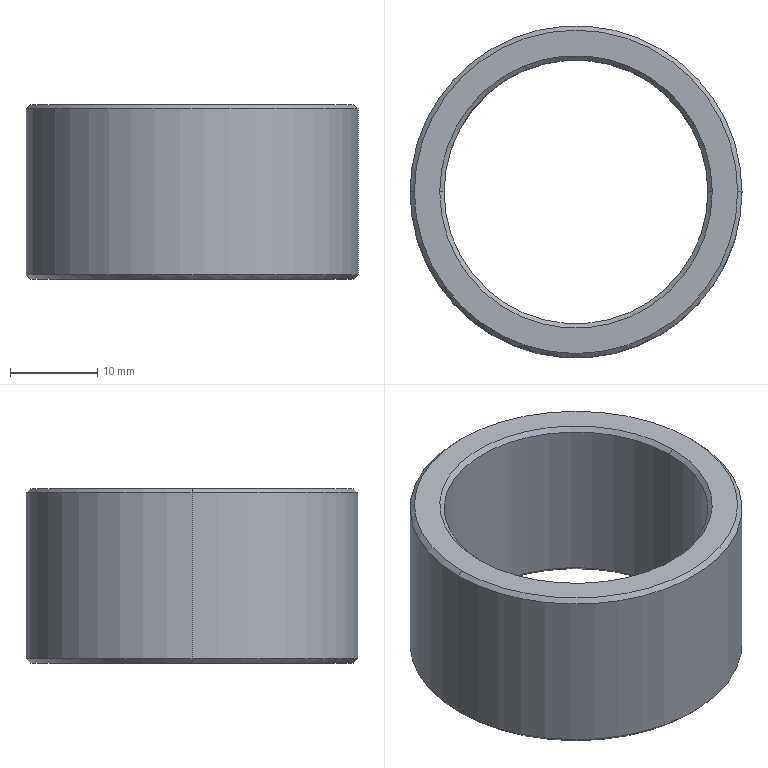Part | STEP file | 2097 Shaft bearing | 1 solid | 14 faces | box 38 x 38 x 20 mm | volume 8302 mm3 | cone 8 | cylinder 4 | plane 2 | commonest cylinder face diameters 30.2 x2 38 x2
STEP:
#1=CARTESIAN_POINT('',(0.,0.,0.));
#2=DIRECTION('',(0.,0.,1.));
#3=DIRECTION('',(1.,0.,0.));
#4=AXIS2_PLACEMENT_3D('',#1,#2,#3);
#5=CARTESIAN_POINT('',(18.5,0.,20.));
#6=VERTEX_POINT('',#5);
#7=CARTESIAN_POINT('',(-18.5,0.,20.));
#8=VERTEX_POINT('',#7);
#9=CARTESIAN_POINT('',(0.,0.,20.));
#10=DIRECTION('',(0.,0.,1.));
#11=DIRECTION('',(1.,0.,0.));
#12=AXIS2_PLACEMENT_3D('',#9,#10,#11);
#13=CIRCLE('',#12,18.5);
#14=CARTESIAN_POINT('',(0.,0.,20.));
#15=DIRECTION('',(0.,0.,-1.));
#16=DIRECTION('',(-1.,0.,0.));
#17=AXIS2_PLACEMENT_3D('',#14,#15,#16);
#18=CONICAL_SURFACE('',#17,18.5,0.7854);
#19=CARTESIAN_POINT('',(3.142,0.));
#20=DIRECTION('',(-1.,0.));
#21=VECTOR('',#20,1.);
#22=LINE('',#19,#21);
#23=(GEOMETRIC_REPRESENTATION_CONTEXT(2)PARAMETRIC_REPRESENTATION_CONTEXT()REPRESENTATION_CONTEXT('',''));
#24=DEFINITIONAL_REPRESENTATION('',(#22),#23);
#25=PCURVE('',#18,#24);
#26=CARTESIAN_POINT('',(0.,0.,20.));
#27=DIRECTION('',(0.,0.,1.));
#28=DIRECTION('',(1.,0.,0.));
#29=AXIS2_PLACEMENT_3D('',#26,#27,#28);
#30=PLANE('',#29);
#31=CARTESIAN_POINT('',(0.,0.));
#32=DIRECTION('',(1.,0.));
#33=AXIS2_PLACEMENT_2D('',#31,#32);
#34=CIRCLE('',#33,18.5);
#35=(GEOMETRIC_REPRESENTATION_CONTEXT(2)PARAMETRIC_REPRESENTATION_CONTEXT()REPRESENTATION_CONTEXT('',''));
#36=DEFINITIONAL_REPRESENTATION('',(#34),#35);
#37=PCURVE('',#30,#36);
#38=SURFACE_CURVE('',#13,(#25,#37),.PCURVE_S1.);
#39=EDGE_CURVE('',#6,#8,#38,.T.);
#40=ORIENTED_EDGE('',*,*,#39,.F.);
#41=CARTESIAN_POINT('',(19.,0.,19.5));
#42=VERTEX_POINT('',#41);
#43=CARTESIAN_POINT('',(18.5,0.,20.));
#44=DIRECTION('',(0.7071,0.,-0.7071));
#45=VECTOR('',#44,1.);
#46=LINE('',#43,#45);
#47=CARTESIAN_POINT('',(3.142,0.));
#48=DIRECTION('',(0.,1.));
#49=VECTOR('',#48,1.);
#50=LINE('',#47,#49);
#51=(GEOMETRIC_REPRESENTATION_CONTEXT(2)PARAMETRIC_REPRESENTATION_CONTEXT()REPRESENTATION_CONTEXT('',''));
#52=DEFINITIONAL_REPRESENTATION('',(#50),#51);
#53=PCURVE('',#18,#52);
#54=CARTESIAN_POINT('',(0.,0.,20.));
#55=DIRECTION('',(0.,0.,-1.));
#56=DIRECTION('',(-1.,0.,0.));
#57=AXIS2_PLACEMENT_3D('',#54,#55,#56);
#58=CONICAL_SURFACE('',#57,18.5,0.7854);
#59=CARTESIAN_POINT('',(3.142,0.));
#60=DIRECTION('',(0.,1.));
#61=VECTOR('',#60,1.);
#62=LINE('',#59,#61);
#63=(GEOMETRIC_REPRESENTATION_CONTEXT(2)PARAMETRIC_REPRESENTATION_CONTEXT()REPRESENTATION_CONTEXT('',''));
#64=DEFINITIONAL_REPRESENTATION('',(#62),#63);
#65=PCURVE('',#58,#64);
#66=SURFACE_CURVE('',#46,(#53,#65),.PCURVE_S1.);
#67=EDGE_CURVE('',#6,#42,#66,.T.);
#68=ORIENTED_EDGE('',*,*,#67,.T.);
#69=CARTESIAN_POINT('',(-19.,0.,19.5));
#70=VERTEX_POINT('',#69);
#71=CARTESIAN_POINT('',(0.,0.,19.5));
#72=DIRECTION('',(0.,0.,-1.));
#73=DIRECTION('',(1.,0.,0.));
#74=AXIS2_PLACEMENT_3D('',#71,#72,#73);
#75=CIRCLE('',#74,19.);
#76=CARTESIAN_POINT('',(-3.142,0.5));
#77=DIRECTION('',(1.,0.));
#78=VECTOR('',#77,1.);
#79=LINE('',#76,#78);
#80=(GEOMETRIC_REPRESENTATION_CONTEXT(2)PARAMETRIC_REPRESENTATION_CONTEXT()REPRESENTATION_CONTEXT('',''));
#81=DEFINITIONAL_REPRESENTATION('',(#79),#80);
#82=PCURVE('',#18,#81);
#83=CARTESIAN_POINT('',(0.,0.,20.));
#84=DIRECTION('',(0.,0.,-1.));
#85=DIRECTION('',(-1.,0.,0.));
#86=AXIS2_PLACEMENT_3D('',#83,#84,#85);
#87=CYLINDRICAL_SURFACE('',#86,19.);
#88=CARTESIAN_POINT('',(-3.142,0.5));
#89=DIRECTION('',(1.,0.));
#90=VECTOR('',#89,1.);
#91=LINE('',#88,#90);
#92=(GEOMETRIC_REPRESENTATION_CONTEXT(2)PARAMETRIC_REPRESENTATION_CONTEXT()REPRESENTATION_CONTEXT('',''));
#93=DEFINITIONAL_REPRESENTATION('',(#91),#92);
#94=PCURVE('',#87,#93);
#95=SURFACE_CURVE('',#75,(#82,#94),.PCURVE_S1.);
#96=EDGE_CURVE('',#70,#42,#95,.T.);
#97=ORIENTED_EDGE('',*,*,#96,.F.);
#98=CARTESIAN_POINT('',(-18.5,0.,20.));
#99=DIRECTION('',(-0.7071,0.,-0.7071));
#100=VECTOR('',#99,1.);
#101=LINE('',#98,#100);
#102=CARTESIAN_POINT('',(0.,0.));
#103=DIRECTION('',(0.,1.));
#104=VECTOR('',#103,1.);
#105=LINE('',#102,#104);
#106=(GEOMETRIC_REPRESENTATION_CONTEXT(2)PARAMETRIC_REPRESENTATION_CONTEXT()REPRESENTATION_CONTEXT('',''));
#107=DEFINITIONAL_REPRESENTATION('',(#105),#106);
#108=PCURVE('',#18,#107);
#109=CARTESIAN_POINT('',(6.283,0.));
#110=DIRECTION('',(0.,1.));
#111=VECTOR('',#110,1.);
#112=LINE('',#109,#111);
#113=(GEOMETRIC_REPRESENTATION_CONTEXT(2)PARAMETRIC_REPRESENTATION_CONTEXT()REPRESENTATION_CONTEXT('',''));
#114=DEFINITIONAL_REPRESENTATION('',(#112),#113);
#115=PCURVE('',#58,#114);
#116=SURFACE_CURVE('',#101,(#108,#115),.PCURVE_S1.);
#117=EDGE_CURVE('',#8,#70,#116,.T.);
#118=ORIENTED_EDGE('',*,*,#117,.F.);
#119=EDGE_LOOP('',(#40,#68,#97,#118));
#120=FACE_BOUND('',#119,.T.);
#121=ADVANCED_FACE('',(#120),#18,.T.);
#122=CARTESIAN_POINT('',(15.1,0.,19.5));
#123=VERTEX_POINT('',#122);
#124=CARTESIAN_POINT('',(15.6,0.,20.));
#125=VERTEX_POINT('',#124);
#126=CARTESIAN_POINT('',(15.1,0.,19.5));
#127=DIRECTION('',(0.7071,0.,0.7071));
#128=VECTOR('',#127,1.);
#129=LINE('',#126,#128);
#130=CARTESIAN_POINT('',(0.,0.,19.5));
#131=DIRECTION('',(0.,0.,1.));
#132=DIRECTION('',(1.,0.,0.));
#133=AXIS2_PLACEMENT_3D('',#130,#131,#132);
#134=CONICAL_SURFACE('',#133,15.1,0.7854);
#135=CARTESIAN_POINT('',(6.283,0.));
#136=DIRECTION('',(0.,1.));
#137=VECTOR('',#136,1.);
#138=LINE('',#135,#137);
#139=(GEOMETRIC_REPRESENTATION_CONTEXT(2)PARAMETRIC_REPRESENTATION_CONTEXT()REPRESENTATION_CONTEXT('',''));
#140=DEFINITIONAL_REPRESENTATION('',(#138),#139);
#141=PCURVE('',#134,#140);
#142=CARTESIAN_POINT('',(0.,0.,19.5));
#143=DIRECTION('',(0.,0.,1.));
#144=DIRECTION('',(1.,0.,0.));
#145=AXIS2_PLACEMENT_3D('',#142,#143,#144);
#146=CONICAL_SURFACE('',#145,15.1,0.7854);
#147=CARTESIAN_POINT('',(0.,0.));
#148=DIRECTION('',(0.,1.));
#149=VECTOR('',#148,1.);
#150=LINE('',#147,#149);
#151=(GEOMETRIC_REPRESENTATION_CONTEXT(2)PARAMETRIC_REPRESENTATION_CONTEXT()REPRESENTATION_CONTEXT('',''));
#152=DEFINITIONAL_REPRESENTATION('',(#150),#151);
#153=PCURVE('',#146,#152);
#154=SURFACE_CURVE('',#129,(#141,#153),.PCURVE_S1.);
#155=EDGE_CURVE('',#123,#125,#154,.T.);
#156=ORIENTED_EDGE('',*,*,#155,.T.);
#157=CARTESIAN_POINT('',(-15.6,0.,20.));
#158=VERTEX_POINT('',#157);
#159=CARTESIAN_POINT('',(0.,0.,20.));
#160=DIRECTION('',(0.,0.,-1.));
#161=DIRECTION('',(1.,0.,0.));
#162=AXIS2_PLACEMENT_3D('',#159,#160,#161);
#163=CIRCLE('',#162,15.6);
#164=CARTESIAN_POINT('',(6.283,0.5));
#165=DIRECTION('',(-1.,0.));
#166=VECTOR('',#165,1.);
#167=LINE('',#164,#166);
#168=(GEOMETRIC_REPRESENTATION_CONTEXT(2)PARAMETRIC_REPRESENTATION_CONTEXT()REPRESENTATION_CONTEXT('',''));
#169=DEFINITIONAL_REPRESENTATION('',(#167),#168);
#170=PCURVE('',#134,#169);
#171=CARTESIAN_POINT('',(15.6,0.));
#172=CARTESIAN_POINT('',(15.6,-27.02));
#173=CARTESIAN_POINT('',(-7.8,-13.51));
#174=CARTESIAN_POINT('',(-31.2,0.));
#175=CARTESIAN_POINT('',(-7.8,13.51));
#176=CARTESIAN_POINT('',(15.6,27.02));
#177=CARTESIAN_POINT('',(15.6,0.));
#178=(BOUNDED_CURVE()B_SPLINE_CURVE(2,(#171,#172,#173,#174,#175,#176,#177),.UNSPECIFIED.,.T.,.F.)B_SPLINE_CURVE_WITH_KNOTS((1,2,2,2,2,1),(-2.094,0.,2.094,4.189,6.283,8.378),.UNSPECIFIED.)CURVE()GEOMETRIC_REPRESENTATION_ITEM()RATIONAL_B_SPLINE_CURVE((1.,0.5,1.,0.5,1.,0.5,1.))REPRESENTATION_ITEM(''));
#179=(GEOMETRIC_REPRESENTATION_CONTEXT(2)PARAMETRIC_REPRESENTATION_CONTEXT()REPRESENTATION_CONTEXT('',''));
#180=DEFINITIONAL_REPRESENTATION('',(#178),#179);
#181=PCURVE('',#30,#180);
#182=SURFACE_CURVE('',#163,(#170,#181),.PCURVE_S1.);
#183=EDGE_CURVE('',#125,#158,#182,.T.);
#184=ORIENTED_EDGE('',*,*,#183,.T.);
#185=CARTESIAN_POINT('',(-15.1,0.,19.5));
#186=VERTEX_POINT('',#185);
#187=CARTESIAN_POINT('',(-15.1,0.,19.5));
#188=DIRECTION('',(-0.7071,0.,0.7071));
#189=VECTOR('',#188,1.);
#190=LINE('',#187,#189);
#191=CARTESIAN_POINT('',(3.142,0.));
#192=DIRECTION('',(0.,1.));
#193=VECTOR('',#192,1.);
#194=LINE('',#191,#193);
#195=(GEOMETRIC_REPRESENTATION_CONTEXT(2)PARAMETRIC_REPRESENTATION_CONTEXT()REPRESENTATION_CONTEXT('',''));
#196=DEFINITIONAL_REPRESENTATION('',(#194),#195);
#197=PCURVE('',#134,#196);
#198=CARTESIAN_POINT('',(3.142,0.));
#199=DIRECTION('',(0.,1.));
#200=VECTOR('',#199,1.);
#201=LINE('',#198,#200);
#202=(GEOMETRIC_REPRESENTATION_CONTEXT(2)PARAMETRIC_REPRESENTATION_CONTEXT()REPRESENTATION_CONTEXT('',''));
#203=DEFINITIONAL_REPRESENTATION('',(#201),#202);
#204=PCURVE('',#146,#203);
#205=SURFACE_CURVE('',#190,(#197,#204),.PCURVE_S1.);
#206=EDGE_CURVE('',#186,#158,#205,.T.);
#207=ORIENTED_EDGE('',*,*,#206,.F.);
#208=CARTESIAN_POINT('',(0.,0.,19.5));
#209=DIRECTION('',(0.,0.,1.));
#210=DIRECTION('',(1.,0.,0.));
#211=AXIS2_PLACEMENT_3D('',#208,#209,#210);
#212=CIRCLE('',#211,15.1);
#213=CARTESIAN_POINT('',(0.,0.));
#214=DIRECTION('',(1.,0.));
#215=VECTOR('',#214,1.);
#216=LINE('',#213,#215);
#217=(GEOMETRIC_REPRESENTATION_CONTEXT(2)PARAMETRIC_REPRESENTATION_CONTEXT()REPRESENTATION_CONTEXT('',''));
#218=DEFINITIONAL_REPRESENTATION('',(#216),#217);
#219=PCURVE('',#134,#218);
#220=CARTESIAN_POINT('',(0.,0.,20.));
#221=DIRECTION('',(0.,0.,-1.));
#222=DIRECTION('',(-1.,0.,0.));
#223=AXIS2_PLACEMENT_3D('',#220,#221,#222);
#224=CYLINDRICAL_SURFACE('',#223,15.1);
#225=CARTESIAN_POINT('',(9.425,0.5));
#226=DIRECTION('',(-1.,0.));
#227=VECTOR('',#226,1.);
#228=LINE('',#225,#227);
#229=(GEOMETRIC_REPRESENTATION_CONTEXT(2)PARAMETRIC_REPRESENTATION_CONTEXT()REPRESENTATION_CONTEXT('',''));
#230=DEFINITIONAL_REPRESENTATION('',(#228),#229);
#231=PCURVE('',#224,#230);
#232=SURFACE_CURVE('',#212,(#219,#231),.PCURVE_S1.);
#233=EDGE_CURVE('',#186,#123,#232,.T.);
#234=ORIENTED_EDGE('',*,*,#233,.T.);
#235=EDGE_LOOP('',(#156,#184,#207,#234));
#236=FACE_BOUND('',#235,.F.);
#237=ADVANCED_FACE('',(#236),#134,.F.);
#238=CARTESIAN_POINT('',(-18.5,0.,0.));
#239=VERTEX_POINT('',#238);
#240=CARTESIAN_POINT('',(18.5,0.,0.));
#241=VERTEX_POINT('',#240);
#242=CARTESIAN_POINT('',(0.,0.,0.));
#243=DIRECTION('',(0.,0.,-1.));
#244=DIRECTION('',(1.,0.,0.));
#245=AXIS2_PLACEMENT_3D('',#242,#243,#244);
#246=CIRCLE('',#245,18.5);
#247=CARTESIAN_POINT('',(0.,0.,0.5));
#248=DIRECTION('',(0.,0.,1.));
#249=DIRECTION('',(1.,0.,0.));
#250=AXIS2_PLACEMENT_3D('',#247,#248,#249);
#251=CONICAL_SURFACE('',#250,19.,0.7854);
#252=CARTESIAN_POINT('',(6.283,-0.5));
#253=DIRECTION('',(-1.,0.));
#254=VECTOR('',#253,1.);
#255=LINE('',#252,#254);
#256=(GEOMETRIC_REPRESENTATION_CONTEXT(2)PARAMETRIC_REPRESENTATION_CONTEXT()REPRESENTATION_CONTEXT('',''));
#257=DEFINITIONAL_REPRESENTATION('',(#255),#256);
#258=PCURVE('',#251,#257);
#259=CARTESIAN_POINT('',(0.,0.,0.));
#260=DIRECTION('',(0.,0.,1.));
#261=DIRECTION('',(1.,0.,0.));
#262=AXIS2_PLACEMENT_3D('',#259,#260,#261);
#263=PLANE('',#262);
#264=CARTESIAN_POINT('',(18.5,0.));
#265=CARTESIAN_POINT('',(18.5,-32.043));
#266=CARTESIAN_POINT('',(-9.25,-16.021));
#267=CARTESIAN_POINT('',(-37.,0.));
#268=CARTESIAN_POINT('',(-9.25,16.021));
#269=CARTESIAN_POINT('',(18.5,32.043));
#270=CARTESIAN_POINT('',(18.5,0.));
#271=(BOUNDED_CURVE()B_SPLINE_CURVE(2,(#264,#265,#266,#267,#268,#269,#270),.UNSPECIFIED.,.T.,.F.)B_SPLINE_CURVE_WITH_KNOTS((1,2,2,2,2,1),(-2.094,0.,2.094,4.189,6.283,8.378),.UNSPECIFIED.)CURVE()GEOMETRIC_REPRESENTATION_ITEM()RATIONAL_B_SPLINE_CURVE((1.,0.5,1.,0.5,1.,0.5,1.))REPRESENTATION_ITEM(''));
#272=(GEOMETRIC_REPRESENTATION_CONTEXT(2)PARAMETRIC_REPRESENTATION_CONTEXT()REPRESENTATION_CONTEXT('',''));
#273=DEFINITIONAL_REPRESENTATION('',(#271),#272);
#274=PCURVE('',#263,#273);
#275=SURFACE_CURVE('',#246,(#258,#274),.PCURVE_S1.);
#276=EDGE_CURVE('',#239,#241,#275,.T.);
#277=ORIENTED_EDGE('',*,*,#276,.F.);
#278=CARTESIAN_POINT('',(-19.,0.,0.5));
#279=VERTEX_POINT('',#278);
#280=CARTESIAN_POINT('',(-19.,0.,0.5));
#281=DIRECTION('',(-0.7071,0.,0.7071));
#282=VECTOR('',#281,1.);
#283=LINE('',#280,#282);
#284=CARTESIAN_POINT('',(3.142,0.));
#285=DIRECTION('',(0.,1.));
#286=VECTOR('',#285,1.);
#287=LINE('',#284,#286);
#288=(GEOMETRIC_REPRESENTATION_CONTEXT(2)PARAMETRIC_REPRESENTATION_CONTEXT()REPRESENTATION_CONTEXT('',''));
#289=DEFINITIONAL_REPRESENTATION('',(#287),#288);
#290=PCURVE('',#251,#289);
#291=CARTESIAN_POINT('',(0.,0.,0.5));
#292=DIRECTION('',(0.,0.,1.));
#293=DIRECTION('',(1.,0.,0.));
#294=AXIS2_PLACEMENT_3D('',#291,#292,#293);
#295=CONICAL_SURFACE('',#294,19.,0.7854);
#296=CARTESIAN_POINT('',(3.142,0.));
#297=DIRECTION('',(0.,1.));
#298=VECTOR('',#297,1.);
#299=LINE('',#296,#298);
#300=(GEOMETRIC_REPRESENTATION_CONTEXT(2)PARAMETRIC_REPRESENTATION_CONTEXT()REPRESENTATION_CONTEXT('',''));
#301=DEFINITIONAL_REPRESENTATION('',(#299),#300);
#302=PCURVE('',#295,#301);
#303=SURFACE_CURVE('',#283,(#290,#302),.PCURVE_S1.);
#304=EDGE_CURVE('',#239,#279,#303,.T.);
#305=ORIENTED_EDGE('',*,*,#304,.T.);
#306=CARTESIAN_POINT('',(19.,0.,0.5));
#307=VERTEX_POINT('',#306);
#308=CARTESIAN_POINT('',(0.,0.,0.5));
#309=DIRECTION('',(0.,0.,1.));
#310=DIRECTION('',(1.,0.,0.));
#311=AXIS2_PLACEMENT_3D('',#308,#309,#310);
#312=CIRCLE('',#311,19.);
#313=CARTESIAN_POINT('',(0.,0.));
#314=DIRECTION('',(1.,0.));
#315=VECTOR('',#314,1.);
#316=LINE('',#313,#315);
#317=(GEOMETRIC_REPRESENTATION_CONTEXT(2)PARAMETRIC_REPRESENTATION_CONTEXT()REPRESENTATION_CONTEXT('',''));
#318=DEFINITIONAL_REPRESENTATION('',(#316),#317);
#319=PCURVE('',#251,#318);
#320=CARTESIAN_POINT('',(3.142,19.5));
#321=DIRECTION('',(-1.,0.));
#322=VECTOR('',#321,1.);
#323=LINE('',#320,#322);
#324=(GEOMETRIC_REPRESENTATION_CONTEXT(2)PARAMETRIC_REPRESENTATION_CONTEXT()REPRESENTATION_CONTEXT('',''));
#325=DEFINITIONAL_REPRESENTATION('',(#323),#324);
#326=PCURVE('',#87,#325);
#327=SURFACE_CURVE('',#312,(#319,#326),.PCURVE_S1.);
#328=EDGE_CURVE('',#307,#279,#327,.T.);
#329=ORIENTED_EDGE('',*,*,#328,.F.);
#330=CARTESIAN_POINT('',(19.,0.,0.5));
#331=DIRECTION('',(0.7071,0.,0.7071));
#332=VECTOR('',#331,1.);
#333=LINE('',#330,#332);
#334=CARTESIAN_POINT('',(0.,0.));
#335=DIRECTION('',(0.,1.));
#336=VECTOR('',#335,1.);
#337=LINE('',#334,#336);
#338=(GEOMETRIC_REPRESENTATION_CONTEXT(2)PARAMETRIC_REPRESENTATION_CONTEXT()REPRESENTATION_CONTEXT('',''));
#339=DEFINITIONAL_REPRESENTATION('',(#337),#338);
#340=PCURVE('',#251,#339);
#341=CARTESIAN_POINT('',(6.283,0.));
#342=DIRECTION('',(0.,1.));
#343=VECTOR('',#342,1.);
#344=LINE('',#341,#343);
#345=(GEOMETRIC_REPRESENTATION_CONTEXT(2)PARAMETRIC_REPRESENTATION_CONTEXT()REPRESENTATION_CONTEXT('',''));
#346=DEFINITIONAL_REPRESENTATION('',(#344),#345);
#347=PCURVE('',#295,#346);
#348=SURFACE_CURVE('',#333,(#340,#347),.PCURVE_S1.);
#349=EDGE_CURVE('',#241,#307,#348,.T.);
#350=ORIENTED_EDGE('',*,*,#349,.F.);
#351=EDGE_LOOP('',(#277,#305,#329,#350));
#352=FACE_BOUND('',#351,.T.);
#353=ADVANCED_FACE('',(#352),#251,.T.);
#354=CARTESIAN_POINT('',(-15.1,0.,0.5));
#355=VERTEX_POINT('',#354);
#356=CARTESIAN_POINT('',(-15.6,0.,0.));
#357=VERTEX_POINT('',#356);
#358=CARTESIAN_POINT('',(-15.6,0.,0.));
#359=DIRECTION('',(-0.7071,0.,-0.7071));
#360=VECTOR('',#359,1.);
#361=LINE('',#358,#360);
#362=CARTESIAN_POINT('',(0.,0.,0.));
#363=DIRECTION('',(0.,0.,-1.));
#364=DIRECTION('',(-1.,0.,0.));
#365=AXIS2_PLACEMENT_3D('',#362,#363,#364);
#366=CONICAL_SURFACE('',#365,15.6,0.7854);
#367=CARTESIAN_POINT('',(6.283,0.));
#368=DIRECTION('',(0.,1.));
#369=VECTOR('',#368,1.);
#370=LINE('',#367,#369);
#371=(GEOMETRIC_REPRESENTATION_CONTEXT(2)PARAMETRIC_REPRESENTATION_CONTEXT()REPRESENTATION_CONTEXT('',''));
#372=DEFINITIONAL_REPRESENTATION('',(#370),#371);
#373=PCURVE('',#366,#372);
#374=CARTESIAN_POINT('',(0.,0.,0.));
#375=DIRECTION('',(0.,0.,-1.));
#376=DIRECTION('',(-1.,0.,0.));
#377=AXIS2_PLACEMENT_3D('',#374,#375,#376);
#378=CONICAL_SURFACE('',#377,15.6,0.7854);
#379=CARTESIAN_POINT('',(0.,0.));
#380=DIRECTION('',(0.,1.));
#381=VECTOR('',#380,1.);
#382=LINE('',#379,#381);
#383=(GEOMETRIC_REPRESENTATION_CONTEXT(2)PARAMETRIC_REPRESENTATION_CONTEXT()REPRESENTATION_CONTEXT('',''));
#384=DEFINITIONAL_REPRESENTATION('',(#382),#383);
#385=PCURVE('',#378,#384);
#386=SURFACE_CURVE('',#361,(#373,#385),.PCURVE_S1.);
#387=EDGE_CURVE('',#355,#357,#386,.T.);
#388=ORIENTED_EDGE('',*,*,#387,.T.);
#389=CARTESIAN_POINT('',(15.6,0.,0.));
#390=VERTEX_POINT('',#389);
#391=CARTESIAN_POINT('',(0.,0.,0.));
#392=DIRECTION('',(0.,0.,1.));
#393=DIRECTION('',(1.,0.,0.));
#394=AXIS2_PLACEMENT_3D('',#391,#392,#393);
#395=CIRCLE('',#394,15.6);
#396=CARTESIAN_POINT('',(9.425,0.));
#397=DIRECTION('',(-1.,0.));
#398=VECTOR('',#397,1.);
#399=LINE('',#396,#398);
#400=(GEOMETRIC_REPRESENTATION_CONTEXT(2)PARAMETRIC_REPRESENTATION_CONTEXT()REPRESENTATION_CONTEXT('',''));
#401=DEFINITIONAL_REPRESENTATION('',(#399),#400);
#402=PCURVE('',#366,#401);
#403=CARTESIAN_POINT('',(0.,0.));
#404=DIRECTION('',(1.,0.));
#405=AXIS2_PLACEMENT_2D('',#403,#404);
#406=CIRCLE('',#405,15.6);
#407=(GEOMETRIC_REPRESENTATION_CONTEXT(2)PARAMETRIC_REPRESENTATION_CONTEXT()REPRESENTATION_CONTEXT('',''));
#408=DEFINITIONAL_REPRESENTATION('',(#406),#407);
#409=PCURVE('',#263,#408);
#410=SURFACE_CURVE('',#395,(#402,#409),.PCURVE_S1.);
#411=EDGE_CURVE('',#357,#390,#410,.T.);
#412=ORIENTED_EDGE('',*,*,#411,.T.);
#413=CARTESIAN_POINT('',(15.1,0.,0.5));
#414=VERTEX_POINT('',#413);
#415=CARTESIAN_POINT('',(15.6,0.,0.));
#416=DIRECTION('',(0.7071,0.,-0.7071));
#417=VECTOR('',#416,1.);
#418=LINE('',#415,#417);
#419=CARTESIAN_POINT('',(3.142,0.));
#420=DIRECTION('',(0.,1.));
#421=VECTOR('',#420,1.);
#422=LINE('',#419,#421);
#423=(GEOMETRIC_REPRESENTATION_CONTEXT(2)PARAMETRIC_REPRESENTATION_CONTEXT()REPRESENTATION_CONTEXT('',''));
#424=DEFINITIONAL_REPRESENTATION('',(#422),#423);
#425=PCURVE('',#366,#424);
#426=CARTESIAN_POINT('',(3.142,0.));
#427=DIRECTION('',(0.,1.));
#428=VECTOR('',#427,1.);
#429=LINE('',#426,#428);
#430=(GEOMETRIC_REPRESENTATION_CONTEXT(2)PARAMETRIC_REPRESENTATION_CONTEXT()REPRESENTATION_CONTEXT('',''));
#431=DEFINITIONAL_REPRESENTATION('',(#429),#430);
#432=PCURVE('',#378,#431);
#433=SURFACE_CURVE('',#418,(#425,#432),.PCURVE_S1.);
#434=EDGE_CURVE('',#414,#390,#433,.T.);
#435=ORIENTED_EDGE('',*,*,#434,.F.);
#436=CARTESIAN_POINT('',(0.,0.,0.5));
#437=DIRECTION('',(0.,0.,-1.));
#438=DIRECTION('',(1.,0.,0.));
#439=AXIS2_PLACEMENT_3D('',#436,#437,#438);
#440=CIRCLE('',#439,15.1);
#441=CARTESIAN_POINT('',(3.142,-0.5));
#442=DIRECTION('',(1.,0.));
#443=VECTOR('',#442,1.);
#444=LINE('',#441,#443);
#445=(GEOMETRIC_REPRESENTATION_CONTEXT(2)PARAMETRIC_REPRESENTATION_CONTEXT()REPRESENTATION_CONTEXT('',''));
#446=DEFINITIONAL_REPRESENTATION('',(#444),#445);
#447=PCURVE('',#366,#446);
#448=CARTESIAN_POINT('',(3.142,19.5));
#449=DIRECTION('',(1.,0.));
#450=VECTOR('',#449,1.);
#451=LINE('',#448,#450);
#452=(GEOMETRIC_REPRESENTATION_CONTEXT(2)PARAMETRIC_REPRESENTATION_CONTEXT()REPRESENTATION_CONTEXT('',''));
#453=DEFINITIONAL_REPRESENTATION('',(#451),#452);
#454=PCURVE('',#224,#453);
#455=SURFACE_CURVE('',#440,(#447,#454),.PCURVE_S1.);
#456=EDGE_CURVE('',#414,#355,#455,.T.);
#457=ORIENTED_EDGE('',*,*,#456,.T.);
#458=EDGE_LOOP('',(#388,#412,#435,#457));
#459=FACE_BOUND('',#458,.F.);
#460=ADVANCED_FACE('',(#459),#366,.F.);
#461=CARTESIAN_POINT('',(-15.1,0.,20.));
#462=DIRECTION('',(0.,0.,-1.));
#463=VECTOR('',#462,1.);
#464=LINE('',#461,#463);
#465=CARTESIAN_POINT('',(6.283,0.));
#466=DIRECTION('',(0.,1.));
#467=VECTOR('',#466,1.);
#468=LINE('',#465,#467);
#469=(GEOMETRIC_REPRESENTATION_CONTEXT(2)PARAMETRIC_REPRESENTATION_CONTEXT()REPRESENTATION_CONTEXT('',''));
#470=DEFINITIONAL_REPRESENTATION('',(#468),#469);
#471=PCURVE('',#224,#470);
#472=CARTESIAN_POINT('',(0.,0.,20.));
#473=DIRECTION('',(0.,0.,-1.));
#474=DIRECTION('',(-1.,0.,0.));
#475=AXIS2_PLACEMENT_3D('',#472,#473,#474);
#476=CYLINDRICAL_SURFACE('',#475,15.1);
#477=CARTESIAN_POINT('',(0.,0.));
#478=DIRECTION('',(0.,1.));
#479=VECTOR('',#478,1.);
#480=LINE('',#477,#479);
#481=(GEOMETRIC_REPRESENTATION_CONTEXT(2)PARAMETRIC_REPRESENTATION_CONTEXT()REPRESENTATION_CONTEXT('',''));
#482=DEFINITIONAL_REPRESENTATION('',(#480),#481);
#483=PCURVE('',#476,#482);
#484=SURFACE_CURVE('',#464,(#471,#483),.PCURVE_S1.);
#485=EDGE_CURVE('',#186,#355,#484,.T.);
#486=ORIENTED_EDGE('',*,*,#485,.T.);
#487=ORIENTED_EDGE('',*,*,#456,.F.);
#488=CARTESIAN_POINT('',(15.1,0.,20.));
#489=DIRECTION('',(0.,0.,-1.));
#490=VECTOR('',#489,1.);
#491=LINE('',#488,#490);
#492=CARTESIAN_POINT('',(3.142,0.));
#493=DIRECTION('',(0.,1.));
#494=VECTOR('',#493,1.);
#495=LINE('',#492,#494);
#496=(GEOMETRIC_REPRESENTATION_CONTEXT(2)PARAMETRIC_REPRESENTATION_CONTEXT()REPRESENTATION_CONTEXT('',''));
#497=DEFINITIONAL_REPRESENTATION('',(#495),#496);
#498=PCURVE('',#224,#497);
#499=CARTESIAN_POINT('',(3.142,0.));
#500=DIRECTION('',(0.,1.));
#501=VECTOR('',#500,1.);
#502=LINE('',#499,#501);
#503=(GEOMETRIC_REPRESENTATION_CONTEXT(2)PARAMETRIC_REPRESENTATION_CONTEXT()REPRESENTATION_CONTEXT('',''));
#504=DEFINITIONAL_REPRESENTATION('',(#502),#503);
#505=PCURVE('',#476,#504);
#506=SURFACE_CURVE('',#491,(#498,#505),.PCURVE_S1.);
#507=EDGE_CURVE('',#123,#414,#506,.T.);
#508=ORIENTED_EDGE('',*,*,#507,.F.);
#509=ORIENTED_EDGE('',*,*,#233,.F.);
#510=EDGE_LOOP('',(#486,#487,#508,#509));
#511=FACE_BOUND('',#510,.F.);
#512=ADVANCED_FACE('',(#511),#224,.F.);
#513=ORIENTED_EDGE('',*,*,#96,.T.);
#514=CARTESIAN_POINT('',(19.,0.,20.));
#515=DIRECTION('',(0.,0.,-1.));
#516=VECTOR('',#515,1.);
#517=LINE('',#514,#516);
#518=CARTESIAN_POINT('',(3.142,0.));
#519=DIRECTION('',(0.,1.));
#520=VECTOR('',#519,1.);
#521=LINE('',#518,#520);
#522=(GEOMETRIC_REPRESENTATION_CONTEXT(2)PARAMETRIC_REPRESENTATION_CONTEXT()REPRESENTATION_CONTEXT('',''));
#523=DEFINITIONAL_REPRESENTATION('',(#521),#522);
#524=PCURVE('',#87,#523);
#525=CARTESIAN_POINT('',(0.,0.,20.));
#526=DIRECTION('',(0.,0.,-1.));
#527=DIRECTION('',(-1.,0.,0.));
#528=AXIS2_PLACEMENT_3D('',#525,#526,#527);
#529=CYLINDRICAL_SURFACE('',#528,19.);
#530=CARTESIAN_POINT('',(3.142,0.));
#531=DIRECTION('',(0.,1.));
#532=VECTOR('',#531,1.);
#533=LINE('',#530,#532);
#534=(GEOMETRIC_REPRESENTATION_CONTEXT(2)PARAMETRIC_REPRESENTATION_CONTEXT()REPRESENTATION_CONTEXT('',''));
#535=DEFINITIONAL_REPRESENTATION('',(#533),#534);
#536=PCURVE('',#529,#535);
#537=SURFACE_CURVE('',#517,(#524,#536),.PCURVE_S1.);
#538=EDGE_CURVE('',#42,#307,#537,.T.);
#539=ORIENTED_EDGE('',*,*,#538,.T.);
#540=ORIENTED_EDGE('',*,*,#328,.T.);
#541=CARTESIAN_POINT('',(-19.,0.,20.));
#542=DIRECTION('',(0.,0.,-1.));
#543=VECTOR('',#542,1.);
#544=LINE('',#541,#543);
#545=CARTESIAN_POINT('',(0.,0.));
#546=DIRECTION('',(0.,1.));
#547=VECTOR('',#546,1.);
#548=LINE('',#545,#547);
#549=(GEOMETRIC_REPRESENTATION_CONTEXT(2)PARAMETRIC_REPRESENTATION_CONTEXT()REPRESENTATION_CONTEXT('',''));
#550=DEFINITIONAL_REPRESENTATION('',(#548),#549);
#551=PCURVE('',#87,#550);
#552=CARTESIAN_POINT('',(6.283,0.));
#553=DIRECTION('',(0.,1.));
#554=VECTOR('',#553,1.);
#555=LINE('',#552,#554);
#556=(GEOMETRIC_REPRESENTATION_CONTEXT(2)PARAMETRIC_REPRESENTATION_CONTEXT()REPRESENTATION_CONTEXT('',''));
#557=DEFINITIONAL_REPRESENTATION('',(#555),#556);
#558=PCURVE('',#529,#557);
#559=SURFACE_CURVE('',#544,(#551,#558),.PCURVE_S1.);
#560=EDGE_CURVE('',#70,#279,#559,.T.);
#561=ORIENTED_EDGE('',*,*,#560,.F.);
#562=EDGE_LOOP('',(#513,#539,#540,#561));
#563=FACE_BOUND('',#562,.T.);
#564=ADVANCED_FACE('',(#563),#87,.T.);
#565=ORIENTED_EDGE('',*,*,#183,.T.);
#566=CARTESIAN_POINT('',(0.,0.,20.));
#567=DIRECTION('',(0.,0.,-1.));
#568=DIRECTION('',(1.,0.,0.));
#569=AXIS2_PLACEMENT_3D('',#566,#567,#568);
#570=CIRCLE('',#569,15.6);
#571=CARTESIAN_POINT('',(15.6,0.));
#572=CARTESIAN_POINT('',(15.6,-27.02));
#573=CARTESIAN_POINT('',(-7.8,-13.51));
#574=CARTESIAN_POINT('',(-31.2,0.));
#575=CARTESIAN_POINT('',(-7.8,13.51));
#576=CARTESIAN_POINT('',(15.6,27.02));
#577=CARTESIAN_POINT('',(15.6,0.));
#578=(BOUNDED_CURVE()B_SPLINE_CURVE(2,(#571,#572,#573,#574,#575,#576,#577),.UNSPECIFIED.,.T.,.F.)B_SPLINE_CURVE_WITH_KNOTS((1,2,2,2,2,1),(-2.094,0.,2.094,4.189,6.283,8.378),.UNSPECIFIED.)CURVE()GEOMETRIC_REPRESENTATION_ITEM()RATIONAL_B_SPLINE_CURVE((1.,0.5,1.,0.5,1.,0.5,1.))REPRESENTATION_ITEM(''));
#579=(GEOMETRIC_REPRESENTATION_CONTEXT(2)PARAMETRIC_REPRESENTATION_CONTEXT()REPRESENTATION_CONTEXT('',''));
#580=DEFINITIONAL_REPRESENTATION('',(#578),#579);
#581=PCURVE('',#30,#580);
#582=CARTESIAN_POINT('',(6.283,0.5));
#583=DIRECTION('',(-1.,0.));
#584=VECTOR('',#583,1.);
#585=LINE('',#582,#584);
#586=(GEOMETRIC_REPRESENTATION_CONTEXT(2)PARAMETRIC_REPRESENTATION_CONTEXT()REPRESENTATION_CONTEXT('',''));
#587=DEFINITIONAL_REPRESENTATION('',(#585),#586);
#588=PCURVE('',#146,#587);
#589=SURFACE_CURVE('',#570,(#581,#588),.PCURVE_S1.);
#590=EDGE_CURVE('',#158,#125,#589,.T.);
#591=ORIENTED_EDGE('',*,*,#590,.T.);
#592=EDGE_LOOP('',(#565,#591));
#593=FACE_BOUND('',#592,.T.);
#594=CARTESIAN_POINT('',(0.,0.,20.));
#595=DIRECTION('',(0.,0.,1.));
#596=DIRECTION('',(1.,0.,0.));
#597=AXIS2_PLACEMENT_3D('',#594,#595,#596);
#598=CIRCLE('',#597,18.5);
#599=CARTESIAN_POINT('',(0.,0.));
#600=DIRECTION('',(1.,0.));
#601=AXIS2_PLACEMENT_2D('',#599,#600);
#602=CIRCLE('',#601,18.5);
#603=(GEOMETRIC_REPRESENTATION_CONTEXT(2)PARAMETRIC_REPRESENTATION_CONTEXT()REPRESENTATION_CONTEXT('',''));
#604=DEFINITIONAL_REPRESENTATION('',(#602),#603);
#605=PCURVE('',#30,#604);
#606=CARTESIAN_POINT('',(9.425,0.));
#607=DIRECTION('',(-1.,0.));
#608=VECTOR('',#607,1.);
#609=LINE('',#606,#608);
#610=(GEOMETRIC_REPRESENTATION_CONTEXT(2)PARAMETRIC_REPRESENTATION_CONTEXT()REPRESENTATION_CONTEXT('',''));
#611=DEFINITIONAL_REPRESENTATION('',(#609),#610);
#612=PCURVE('',#58,#611);
#613=SURFACE_CURVE('',#598,(#605,#612),.PCURVE_S1.);
#614=EDGE_CURVE('',#8,#6,#613,.T.);
#615=ORIENTED_EDGE('',*,*,#614,.T.);
#616=ORIENTED_EDGE('',*,*,#39,.T.);
#617=EDGE_LOOP('',(#615,#616));
#618=FACE_BOUND('',#617,.T.);
#619=ADVANCED_FACE('',(#593,#618),#30,.T.);
#620=ORIENTED_EDGE('',*,*,#411,.T.);
#621=CARTESIAN_POINT('',(0.,0.,0.));
#622=DIRECTION('',(0.,0.,1.));
#623=DIRECTION('',(1.,0.,0.));
#624=AXIS2_PLACEMENT_3D('',#621,#622,#623);
#625=CIRCLE('',#624,15.6);
#626=CARTESIAN_POINT('',(0.,0.));
#627=DIRECTION('',(1.,0.));
#628=AXIS2_PLACEMENT_2D('',#626,#627);
#629=CIRCLE('',#628,15.6);
#630=(GEOMETRIC_REPRESENTATION_CONTEXT(2)PARAMETRIC_REPRESENTATION_CONTEXT()REPRESENTATION_CONTEXT('',''));
#631=DEFINITIONAL_REPRESENTATION('',(#629),#630);
#632=PCURVE('',#263,#631);
#633=CARTESIAN_POINT('',(3.142,0.));
#634=DIRECTION('',(-1.,0.));
#635=VECTOR('',#634,1.);
#636=LINE('',#633,#635);
#637=(GEOMETRIC_REPRESENTATION_CONTEXT(2)PARAMETRIC_REPRESENTATION_CONTEXT()REPRESENTATION_CONTEXT('',''));
#638=DEFINITIONAL_REPRESENTATION('',(#636),#637);
#639=PCURVE('',#378,#638);
#640=SURFACE_CURVE('',#625,(#632,#639),.PCURVE_S1.);
#641=EDGE_CURVE('',#390,#357,#640,.T.);
#642=ORIENTED_EDGE('',*,*,#641,.T.);
#643=EDGE_LOOP('',(#620,#642));
#644=FACE_BOUND('',#643,.T.);
#645=CARTESIAN_POINT('',(0.,0.,0.));
#646=DIRECTION('',(0.,0.,-1.));
#647=DIRECTION('',(1.,0.,0.));
#648=AXIS2_PLACEMENT_3D('',#645,#646,#647);
#649=CIRCLE('',#648,18.5);
#650=CARTESIAN_POINT('',(18.5,0.));
#651=CARTESIAN_POINT('',(18.5,-32.043));
#652=CARTESIAN_POINT('',(-9.25,-16.021));
#653=CARTESIAN_POINT('',(-37.,0.));
#654=CARTESIAN_POINT('',(-9.25,16.021));
#655=CARTESIAN_POINT('',(18.5,32.043));
#656=CARTESIAN_POINT('',(18.5,0.));
#657=(BOUNDED_CURVE()B_SPLINE_CURVE(2,(#650,#651,#652,#653,#654,#655,#656),.UNSPECIFIED.,.T.,.F.)B_SPLINE_CURVE_WITH_KNOTS((1,2,2,2,2,1),(-2.094,0.,2.094,4.189,6.283,8.378),.UNSPECIFIED.)CURVE()GEOMETRIC_REPRESENTATION_ITEM()RATIONAL_B_SPLINE_CURVE((1.,0.5,1.,0.5,1.,0.5,1.))REPRESENTATION_ITEM(''));
#658=(GEOMETRIC_REPRESENTATION_CONTEXT(2)PARAMETRIC_REPRESENTATION_CONTEXT()REPRESENTATION_CONTEXT('',''));
#659=DEFINITIONAL_REPRESENTATION('',(#657),#658);
#660=PCURVE('',#263,#659);
#661=CARTESIAN_POINT('',(6.283,-0.5));
#662=DIRECTION('',(-1.,0.));
#663=VECTOR('',#662,1.);
#664=LINE('',#661,#663);
#665=(GEOMETRIC_REPRESENTATION_CONTEXT(2)PARAMETRIC_REPRESENTATION_CONTEXT()REPRESENTATION_CONTEXT('',''));
#666=DEFINITIONAL_REPRESENTATION('',(#664),#665);
#667=PCURVE('',#295,#666);
#668=SURFACE_CURVE('',#649,(#660,#667),.PCURVE_S1.);
#669=EDGE_CURVE('',#241,#239,#668,.T.);
#670=ORIENTED_EDGE('',*,*,#669,.T.);
#671=ORIENTED_EDGE('',*,*,#276,.T.);
#672=EDGE_LOOP('',(#670,#671));
#673=FACE_BOUND('',#672,.T.);
#674=ADVANCED_FACE('',(#644,#673),#263,.F.);
#675=ORIENTED_EDGE('',*,*,#538,.F.);
#676=CARTESIAN_POINT('',(0.,0.,19.5));
#677=DIRECTION('',(0.,0.,-1.));
#678=DIRECTION('',(1.,0.,0.));
#679=AXIS2_PLACEMENT_3D('',#676,#677,#678);
#680=CIRCLE('',#679,19.);
#681=CARTESIAN_POINT('',(3.142,0.5));
#682=DIRECTION('',(1.,0.));
#683=VECTOR('',#682,1.);
#684=LINE('',#681,#683);
#685=(GEOMETRIC_REPRESENTATION_CONTEXT(2)PARAMETRIC_REPRESENTATION_CONTEXT()REPRESENTATION_CONTEXT('',''));
#686=DEFINITIONAL_REPRESENTATION('',(#684),#685);
#687=PCURVE('',#529,#686);
#688=CARTESIAN_POINT('',(3.142,0.5));
#689=DIRECTION('',(1.,0.));
#690=VECTOR('',#689,1.);
#691=LINE('',#688,#690);
#692=(GEOMETRIC_REPRESENTATION_CONTEXT(2)PARAMETRIC_REPRESENTATION_CONTEXT()REPRESENTATION_CONTEXT('',''));
#693=DEFINITIONAL_REPRESENTATION('',(#691),#692);
#694=PCURVE('',#58,#693);
#695=SURFACE_CURVE('',#680,(#687,#694),.PCURVE_S1.);
#696=EDGE_CURVE('',#42,#70,#695,.T.);
#697=ORIENTED_EDGE('',*,*,#696,.T.);
#698=ORIENTED_EDGE('',*,*,#560,.T.);
#699=CARTESIAN_POINT('',(0.,0.,0.5));
#700=DIRECTION('',(0.,0.,1.));
#701=DIRECTION('',(1.,0.,0.));
#702=AXIS2_PLACEMENT_3D('',#699,#700,#701);
#703=CIRCLE('',#702,19.);
#704=CARTESIAN_POINT('',(9.425,19.5));
#705=DIRECTION('',(-1.,0.));
#706=VECTOR('',#705,1.);
#707=LINE('',#704,#706);
#708=(GEOMETRIC_REPRESENTATION_CONTEXT(2)PARAMETRIC_REPRESENTATION_CONTEXT()REPRESENTATION_CONTEXT('',''));
#709=DEFINITIONAL_REPRESENTATION('',(#707),#708);
#710=PCURVE('',#529,#709);
#711=CARTESIAN_POINT('',(0.,0.));
#712=DIRECTION('',(1.,0.));
#713=VECTOR('',#712,1.);
#714=LINE('',#711,#713);
#715=(GEOMETRIC_REPRESENTATION_CONTEXT(2)PARAMETRIC_REPRESENTATION_CONTEXT()REPRESENTATION_CONTEXT('',''));
#716=DEFINITIONAL_REPRESENTATION('',(#714),#715);
#717=PCURVE('',#295,#716);
#718=SURFACE_CURVE('',#703,(#710,#717),.PCURVE_S1.);
#719=EDGE_CURVE('',#279,#307,#718,.T.);
#720=ORIENTED_EDGE('',*,*,#719,.T.);
#721=EDGE_LOOP('',(#675,#697,#698,#720));
#722=FACE_BOUND('',#721,.T.);
#723=ADVANCED_FACE('',(#722),#529,.T.);
#724=CARTESIAN_POINT('',(0.,0.,0.5));
#725=DIRECTION('',(0.,0.,-1.));
#726=DIRECTION('',(1.,0.,0.));
#727=AXIS2_PLACEMENT_3D('',#724,#725,#726);
#728=CIRCLE('',#727,15.1);
#729=CARTESIAN_POINT('',(-3.142,19.5));
#730=DIRECTION('',(1.,0.));
#731=VECTOR('',#730,1.);
#732=LINE('',#729,#731);
#733=(GEOMETRIC_REPRESENTATION_CONTEXT(2)PARAMETRIC_REPRESENTATION_CONTEXT()REPRESENTATION_CONTEXT('',''));
#734=DEFINITIONAL_REPRESENTATION('',(#732),#733);
#735=PCURVE('',#476,#734);
#736=CARTESIAN_POINT('',(-3.142,-0.5));
#737=DIRECTION('',(1.,0.));
#738=VECTOR('',#737,1.);
#739=LINE('',#736,#738);
#740=(GEOMETRIC_REPRESENTATION_CONTEXT(2)PARAMETRIC_REPRESENTATION_CONTEXT()REPRESENTATION_CONTEXT('',''));
#741=DEFINITIONAL_REPRESENTATION('',(#739),#740);
#742=PCURVE('',#378,#741);
#743=SURFACE_CURVE('',#728,(#735,#742),.PCURVE_S1.);
#744=EDGE_CURVE('',#355,#414,#743,.T.);
#745=ORIENTED_EDGE('',*,*,#744,.F.);
#746=ORIENTED_EDGE('',*,*,#485,.F.);
#747=CARTESIAN_POINT('',(0.,0.,19.5));
#748=DIRECTION('',(0.,0.,1.));
#749=DIRECTION('',(1.,0.,0.));
#750=AXIS2_PLACEMENT_3D('',#747,#748,#749);
#751=CIRCLE('',#750,15.1);
#752=CARTESIAN_POINT('',(3.142,0.5));
#753=DIRECTION('',(-1.,0.));
#754=VECTOR('',#753,1.);
#755=LINE('',#752,#754);
#756=(GEOMETRIC_REPRESENTATION_CONTEXT(2)PARAMETRIC_REPRESENTATION_CONTEXT()REPRESENTATION_CONTEXT('',''));
#757=DEFINITIONAL_REPRESENTATION('',(#755),#756);
#758=PCURVE('',#476,#757);
#759=CARTESIAN_POINT('',(0.,0.));
#760=DIRECTION('',(1.,0.));
#761=VECTOR('',#760,1.);
#762=LINE('',#759,#761);
#763=(GEOMETRIC_REPRESENTATION_CONTEXT(2)PARAMETRIC_REPRESENTATION_CONTEXT()REPRESENTATION_CONTEXT('',''));
#764=DEFINITIONAL_REPRESENTATION('',(#762),#763);
#765=PCURVE('',#146,#764);
#766=SURFACE_CURVE('',#751,(#758,#765),.PCURVE_S1.);
#767=EDGE_CURVE('',#123,#186,#766,.T.);
#768=ORIENTED_EDGE('',*,*,#767,.F.);
#769=ORIENTED_EDGE('',*,*,#507,.T.);
#770=EDGE_LOOP('',(#745,#746,#768,#769));
#771=FACE_BOUND('',#770,.F.);
#772=ADVANCED_FACE('',(#771),#476,.F.);
#773=ORIENTED_EDGE('',*,*,#641,.T.);
#774=ORIENTED_EDGE('',*,*,#387,.F.);
#775=ORIENTED_EDGE('',*,*,#744,.T.);
#776=ORIENTED_EDGE('',*,*,#434,.T.);
#777=EDGE_LOOP('',(#773,#774,#775,#776));
#778=FACE_BOUND('',#777,.F.);
#779=ADVANCED_FACE('',(#778),#378,.F.);
#780=ORIENTED_EDGE('',*,*,#304,.F.);
#781=ORIENTED_EDGE('',*,*,#669,.F.);
#782=ORIENTED_EDGE('',*,*,#349,.T.);
#783=ORIENTED_EDGE('',*,*,#719,.F.);
#784=EDGE_LOOP('',(#780,#781,#782,#783));
#785=FACE_BOUND('',#784,.T.);
#786=ADVANCED_FACE('',(#785),#295,.T.);
#787=ORIENTED_EDGE('',*,*,#590,.T.);
#788=ORIENTED_EDGE('',*,*,#155,.F.);
#789=ORIENTED_EDGE('',*,*,#767,.T.);
#790=ORIENTED_EDGE('',*,*,#206,.T.);
#791=EDGE_LOOP('',(#787,#788,#789,#790));
#792=FACE_BOUND('',#791,.F.);
#793=ADVANCED_FACE('',(#792),#146,.F.);
#794=ORIENTED_EDGE('',*,*,#67,.F.);
#795=ORIENTED_EDGE('',*,*,#614,.F.);
#796=ORIENTED_EDGE('',*,*,#117,.T.);
#797=ORIENTED_EDGE('',*,*,#696,.F.);
#798=EDGE_LOOP('',(#794,#795,#796,#797));
#799=FACE_BOUND('',#798,.T.);
#800=ADVANCED_FACE('',(#799),#58,.T.);
#801=CLOSED_SHELL('',(#121,#237,#353,#460,#512,#564,#619,#674,#723,#772,#779,#786,#793,#800));
#802=MANIFOLD_SOLID_BREP('',#801);
#803=(LENGTH_UNIT()NAMED_UNIT(*)SI_UNIT(.MILLI.,.METRE.));
#804=UNCERTAINTY_MEASURE_WITH_UNIT(LENGTH_MEASURE(0.0000001),#803,'','');
#805=(NAMED_UNIT(*)PLANE_ANGLE_UNIT()SI_UNIT($,.RADIAN.));
#806=(NAMED_UNIT(*)SI_UNIT($,.STERADIAN.)SOLID_ANGLE_UNIT());
#807=(GEOMETRIC_REPRESENTATION_CONTEXT(3)GLOBAL_UNCERTAINTY_ASSIGNED_CONTEXT((#804))GLOBAL_UNIT_ASSIGNED_CONTEXT((#803,#805,#806))REPRESENTATION_CONTEXT('',''));
#808=ADVANCED_BREP_SHAPE_REPRESENTATION('',(#4,#802),#807);